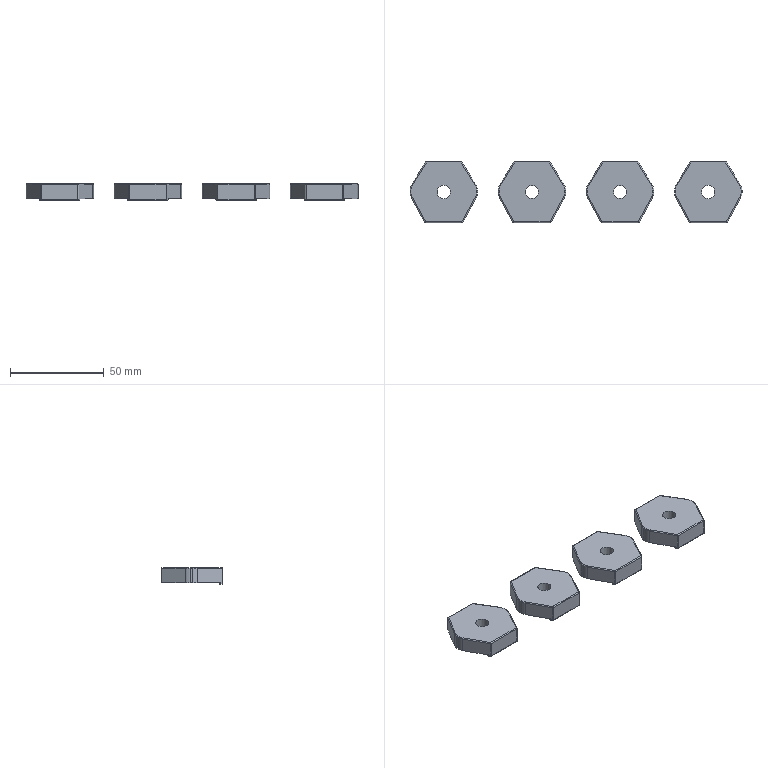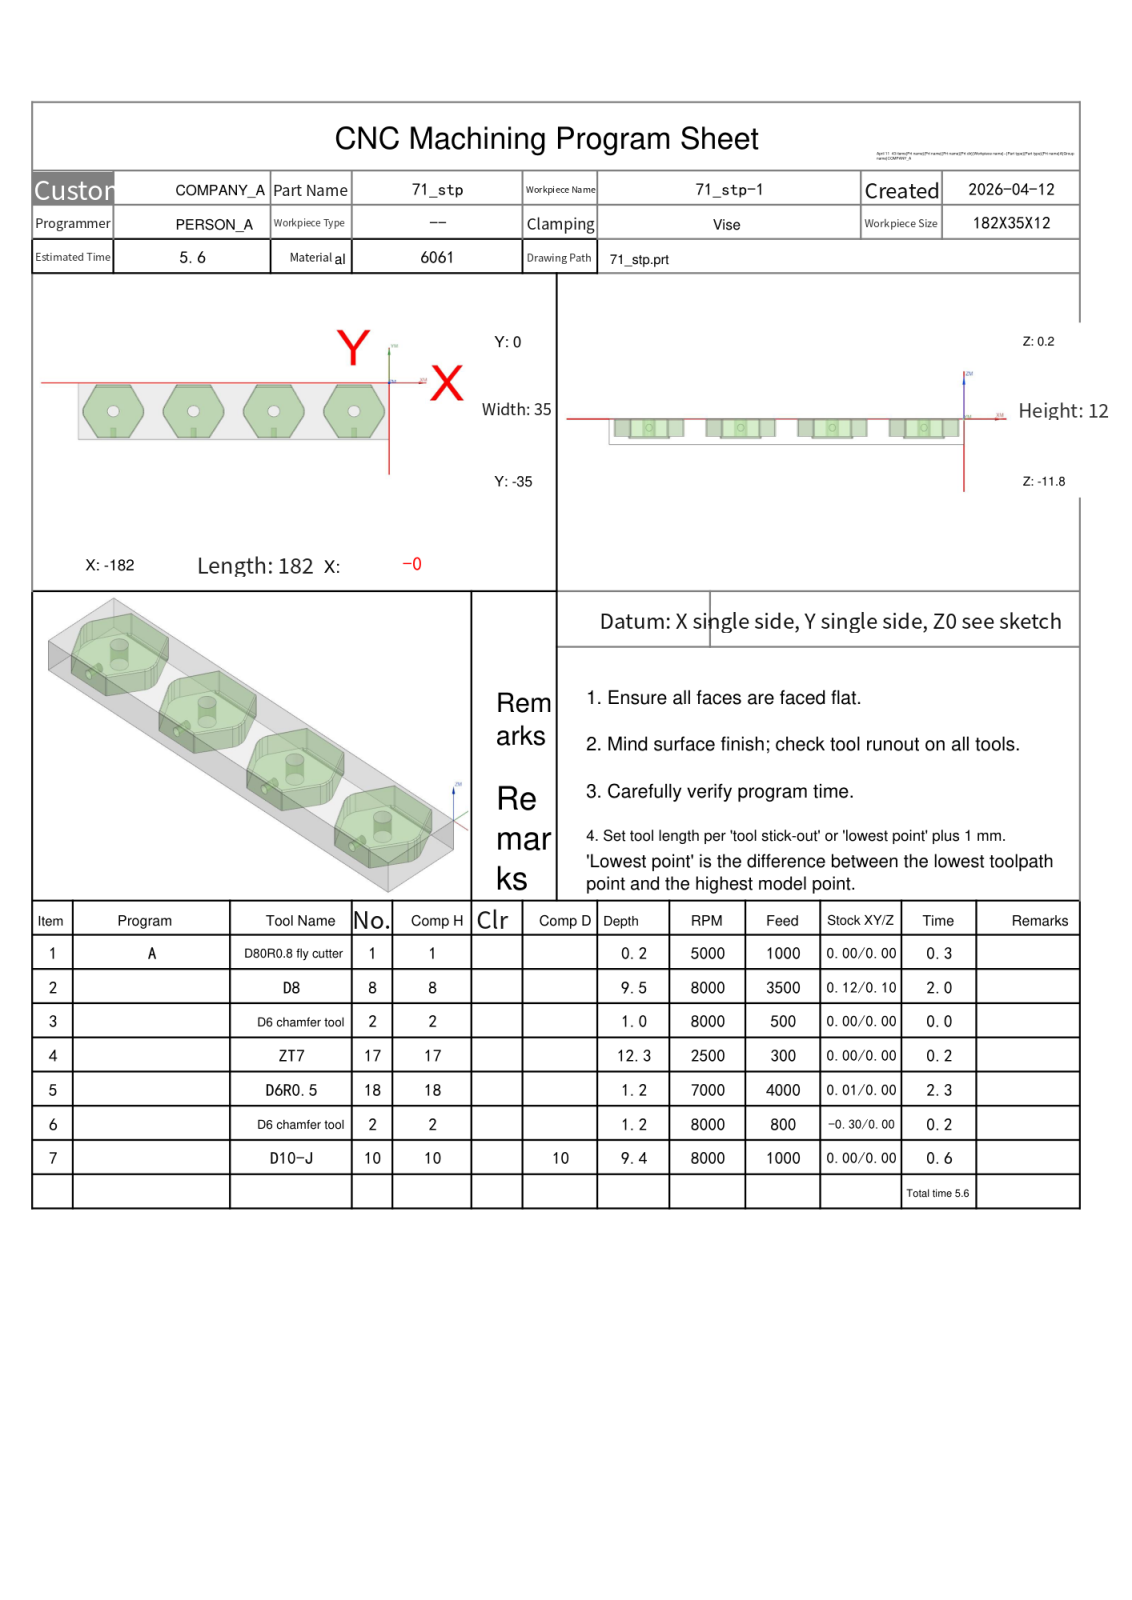NC program | NX | posted by the shop | part box 177 x 33 x 9 mm
Lines 3080 to 3113 of 15773:
N3 T02 M06
(D6 chamfer tool  D=6. R=0. H=02 ce=0.00 di=0.10)
(MAX_Z=20. MIN_Z=-0.8 Time=0.04M)
G00 G90 G54 X-20.5 Y-17.5 M03 S8000
G43 H02 Z20.
M08
G98 G81 X-20.5 Y-17.5 Z-.8 R1. F500.
X-67.5
X-114.5
X-161.5
G80
G00 Z20.
G91 G28 Z0.0
M05
M09
G91 G28 Z0.0
M01
N4 T17 M06
(ZT7 D=7. DR_a=118 H=17)
(MAX_Z=20. MIN_Z=-12.1 Time=0.20M)
G00 G90 G54 X-20.5 Y-17.5 M03 S2500
G43 H17 Z20.
M08
G98 G83 X-20.5 Y-17.5 Z-12.103 R1. F300. Q3.
X-67.5
X-114.5
X-161.5
G80
G00 Z20.
G91 G28 Z0.0
M05
M09
G91 G28 Z0.0
M01